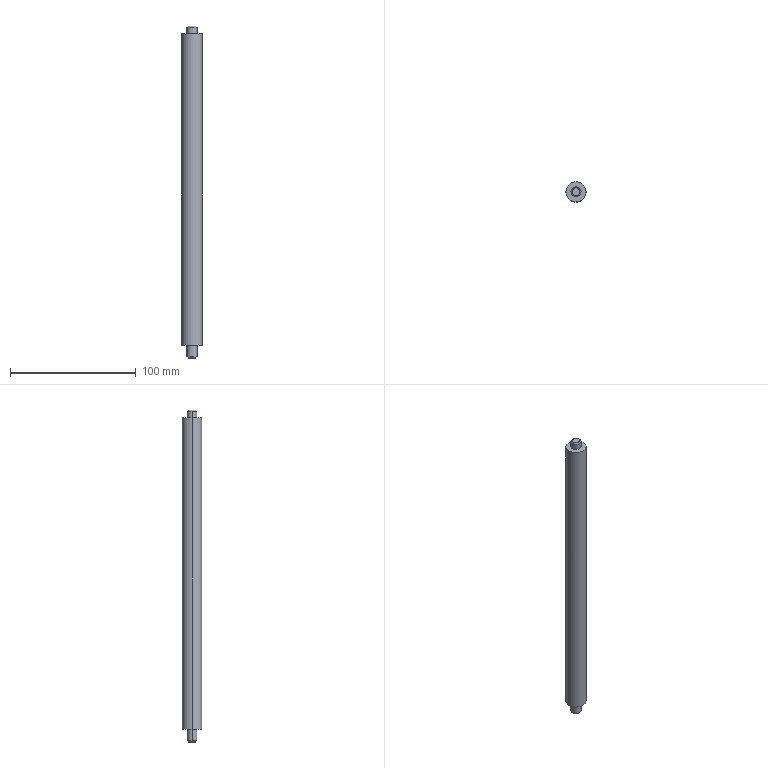Part | SolidWorks | features ICE 2, Chamfer 1, Extrusion 1, Helix 1 | 1 solid | 14 faces | box 16 x 16 x 264 mm | volume 50645 mm3 | cylinder 6 | cone 4 | plane 4 | commonest cylinder face diameters 8 x4 16 x2
STEP:
#1=CARTESIAN_POINT('',(3.,0.,254.));
#2=VERTEX_POINT('',#1);
#3=CARTESIAN_POINT('',(-3.,0.,254.));
#4=VERTEX_POINT('',#3);
#5=CARTESIAN_POINT('',(0.,0.,254.));
#6=DIRECTION('',(0.,0.,1.));
#7=DIRECTION('',(1.,0.,0.));
#8=AXIS2_PLACEMENT_3D('',#5,#6,#7);
#9=CIRCLE('',#8,3.);
#10=EDGE_CURVE('',#2,#4,#9,.T.);
#11=ORIENTED_EDGE('',*,*,#10,.F.);
#12=CARTESIAN_POINT('',(4.,0.,253.));
#13=VERTEX_POINT('',#12);
#14=CARTESIAN_POINT('',(3.,0.,254.));
#15=DIRECTION('',(0.7071,0.,-0.7071));
#16=VECTOR('',#15,1000.);
#17=LINE('',#14,#16);
#18=EDGE_CURVE('',#2,#13,#17,.T.);
#19=ORIENTED_EDGE('',*,*,#18,.T.);
#20=CARTESIAN_POINT('',(-4.,0.,253.));
#21=VERTEX_POINT('',#20);
#22=CARTESIAN_POINT('',(0.,0.,253.));
#23=DIRECTION('',(0.,0.,-1.));
#24=DIRECTION('',(1.,0.,0.));
#25=AXIS2_PLACEMENT_3D('',#22,#23,#24);
#26=CIRCLE('',#25,4.);
#27=EDGE_CURVE('',#21,#13,#26,.T.);
#28=ORIENTED_EDGE('',*,*,#27,.F.);
#29=CARTESIAN_POINT('',(-3.,0.,254.));
#30=DIRECTION('',(-0.7071,0.,-0.7071));
#31=VECTOR('',#30,1000.);
#32=LINE('',#29,#31);
#33=EDGE_CURVE('',#4,#21,#32,.T.);
#34=ORIENTED_EDGE('',*,*,#33,.F.);
#35=EDGE_LOOP('',(#11,#19,#28,#34));
#36=FACE_OUTER_BOUND('',#35,.T.);
#37=CARTESIAN_POINT('',(0.,0.,254.));
#38=DIRECTION('',(0.,0.,-1.));
#39=DIRECTION('',(-1.,0.,0.));
#40=AXIS2_PLACEMENT_3D('',#37,#38,#39);
#41=CONICAL_SURFACE('',#40,3.,0.7854);
#42=ADVANCED_FACE('',(#36),#41,.T.);
#43=CARTESIAN_POINT('',(-3.,0.,-10.));
#44=VERTEX_POINT('',#43);
#45=CARTESIAN_POINT('',(3.,0.,-10.));
#46=VERTEX_POINT('',#45);
#47=CARTESIAN_POINT('',(0.,0.,-10.));
#48=DIRECTION('',(0.,0.,-1.));
#49=DIRECTION('',(-1.,0.,0.));
#50=AXIS2_PLACEMENT_3D('',#47,#48,#49);
#51=CIRCLE('',#50,3.);
#52=EDGE_CURVE('',#44,#46,#51,.T.);
#53=ORIENTED_EDGE('',*,*,#52,.F.);
#54=CARTESIAN_POINT('',(-4.,0.,-9.));
#55=VERTEX_POINT('',#54);
#56=CARTESIAN_POINT('',(-3.,0.,-10.));
#57=DIRECTION('',(-0.7071,0.,0.7071));
#58=VECTOR('',#57,1000.);
#59=LINE('',#56,#58);
#60=EDGE_CURVE('',#44,#55,#59,.T.);
#61=ORIENTED_EDGE('',*,*,#60,.T.);
#62=CARTESIAN_POINT('',(4.,0.,-9.));
#63=VERTEX_POINT('',#62);
#64=CARTESIAN_POINT('',(0.,0.,-9.));
#65=DIRECTION('',(0.,0.,1.));
#66=DIRECTION('',(-1.,0.,0.));
#67=AXIS2_PLACEMENT_3D('',#64,#65,#66);
#68=CIRCLE('',#67,4.);
#69=EDGE_CURVE('',#63,#55,#68,.T.);
#70=ORIENTED_EDGE('',*,*,#69,.F.);
#71=CARTESIAN_POINT('',(3.,0.,-10.));
#72=DIRECTION('',(0.7071,0.,0.7071));
#73=VECTOR('',#72,1000.);
#74=LINE('',#71,#73);
#75=EDGE_CURVE('',#46,#63,#74,.T.);
#76=ORIENTED_EDGE('',*,*,#75,.F.);
#77=EDGE_LOOP('',(#53,#61,#70,#76));
#78=FACE_OUTER_BOUND('',#77,.T.);
#79=CARTESIAN_POINT('',(0.,0.,-10.));
#80=DIRECTION('',(0.,0.,1.));
#81=DIRECTION('',(1.,0.,0.));
#82=AXIS2_PLACEMENT_3D('',#79,#80,#81);
#83=CONICAL_SURFACE('',#82,3.,0.7854);
#84=ADVANCED_FACE('',(#78),#83,.T.);
#85=ORIENTED_EDGE('',*,*,#27,.T.);
#86=CARTESIAN_POINT('',(4.,0.,248.));
#87=VERTEX_POINT('',#86);
#88=CARTESIAN_POINT('',(4.,0.,254.));
#89=DIRECTION('',(0.,0.,-1.));
#90=VECTOR('',#89,1000.);
#91=LINE('',#88,#90);
#92=EDGE_CURVE('',#13,#87,#91,.T.);
#93=ORIENTED_EDGE('',*,*,#92,.T.);
#94=CARTESIAN_POINT('',(-4.,0.,248.));
#95=VERTEX_POINT('',#94);
#96=CARTESIAN_POINT('',(0.,0.,248.));
#97=DIRECTION('',(0.,0.,1.));
#98=DIRECTION('',(1.,0.,0.));
#99=AXIS2_PLACEMENT_3D('',#96,#97,#98);
#100=CIRCLE('',#99,4.);
#101=EDGE_CURVE('',#87,#95,#100,.T.);
#102=ORIENTED_EDGE('',*,*,#101,.T.);
#103=CARTESIAN_POINT('',(-4.,0.,254.));
#104=DIRECTION('',(0.,0.,-1.));
#105=VECTOR('',#104,1000.);
#106=LINE('',#103,#105);
#107=EDGE_CURVE('',#21,#95,#106,.T.);
#108=ORIENTED_EDGE('',*,*,#107,.F.);
#109=EDGE_LOOP('',(#85,#93,#102,#108));
#110=FACE_OUTER_BOUND('',#109,.T.);
#111=CARTESIAN_POINT('',(0.,0.,254.));
#112=DIRECTION('',(0.,0.,-1.));
#113=DIRECTION('',(-1.,0.,0.));
#114=AXIS2_PLACEMENT_3D('',#111,#112,#113);
#115=CYLINDRICAL_SURFACE('',#114,4.);
#116=ADVANCED_FACE('',(#110),#115,.T.);
#117=ORIENTED_EDGE('',*,*,#69,.T.);
#118=CARTESIAN_POINT('',(-4.,0.,0.));
#119=VERTEX_POINT('',#118);
#120=CARTESIAN_POINT('',(-4.,0.,-10.));
#121=DIRECTION('',(0.,0.,1.));
#122=VECTOR('',#121,1000.);
#123=LINE('',#120,#122);
#124=EDGE_CURVE('',#55,#119,#123,.T.);
#125=ORIENTED_EDGE('',*,*,#124,.T.);
#126=CARTESIAN_POINT('',(4.,0.,0.));
#127=VERTEX_POINT('',#126);
#128=CARTESIAN_POINT('',(0.,0.,0.));
#129=DIRECTION('',(0.,0.,-1.));
#130=DIRECTION('',(1.,0.,0.));
#131=AXIS2_PLACEMENT_3D('',#128,#129,#130);
#132=CIRCLE('',#131,4.);
#133=EDGE_CURVE('',#119,#127,#132,.T.);
#134=ORIENTED_EDGE('',*,*,#133,.T.);
#135=CARTESIAN_POINT('',(4.,0.,-10.));
#136=DIRECTION('',(0.,0.,1.));
#137=VECTOR('',#136,1000.);
#138=LINE('',#135,#137);
#139=EDGE_CURVE('',#63,#127,#138,.T.);
#140=ORIENTED_EDGE('',*,*,#139,.F.);
#141=EDGE_LOOP('',(#117,#125,#134,#140));
#142=FACE_OUTER_BOUND('',#141,.T.);
#143=CARTESIAN_POINT('',(0.,0.,-10.));
#144=DIRECTION('',(0.,0.,1.));
#145=DIRECTION('',(1.,0.,0.));
#146=AXIS2_PLACEMENT_3D('',#143,#144,#145);
#147=CYLINDRICAL_SURFACE('',#146,4.);
#148=ADVANCED_FACE('',(#142),#147,.T.);
#149=CARTESIAN_POINT('',(8.,0.,248.));
#150=VERTEX_POINT('',#149);
#151=CARTESIAN_POINT('',(-8.,0.,248.));
#152=VERTEX_POINT('',#151);
#153=CARTESIAN_POINT('',(0.,0.,248.));
#154=DIRECTION('',(0.,0.,1.));
#155=DIRECTION('',(1.,0.,0.));
#156=AXIS2_PLACEMENT_3D('',#153,#154,#155);
#157=CIRCLE('',#156,8.);
#158=EDGE_CURVE('',#150,#152,#157,.T.);
#159=ORIENTED_EDGE('',*,*,#158,.F.);
#160=CARTESIAN_POINT('',(8.,0.,0.));
#161=VERTEX_POINT('',#160);
#162=CARTESIAN_POINT('',(8.,0.,248.));
#163=DIRECTION('',(0.,0.,-1.));
#164=VECTOR('',#163,1000.);
#165=LINE('',#162,#164);
#166=EDGE_CURVE('',#150,#161,#165,.T.);
#167=ORIENTED_EDGE('',*,*,#166,.T.);
#168=CARTESIAN_POINT('',(-8.,0.,0.));
#169=VERTEX_POINT('',#168);
#170=CARTESIAN_POINT('',(0.,0.,0.));
#171=DIRECTION('',(0.,0.,1.));
#172=DIRECTION('',(1.,0.,0.));
#173=AXIS2_PLACEMENT_3D('',#170,#171,#172);
#174=CIRCLE('',#173,8.);
#175=EDGE_CURVE('',#161,#169,#174,.T.);
#176=ORIENTED_EDGE('',*,*,#175,.T.);
#177=CARTESIAN_POINT('',(-8.,0.,248.));
#178=DIRECTION('',(0.,0.,-1.));
#179=VECTOR('',#178,1000.);
#180=LINE('',#177,#179);
#181=EDGE_CURVE('',#152,#169,#180,.T.);
#182=ORIENTED_EDGE('',*,*,#181,.F.);
#183=EDGE_LOOP('',(#159,#167,#176,#182));
#184=FACE_OUTER_BOUND('',#183,.T.);
#185=CARTESIAN_POINT('',(0.,0.,248.));
#186=DIRECTION('',(0.,0.,-1.));
#187=DIRECTION('',(-1.,0.,0.));
#188=AXIS2_PLACEMENT_3D('',#185,#186,#187);
#189=CYLINDRICAL_SURFACE('',#188,8.);
#190=ADVANCED_FACE('',(#184),#189,.T.);
#191=CARTESIAN_POINT('',(0.,0.,248.));
#192=DIRECTION('',(0.,0.,1.));
#193=DIRECTION('',(1.,0.,0.));
#194=AXIS2_PLACEMENT_3D('',#191,#192,#193);
#195=CIRCLE('',#194,8.);
#196=EDGE_CURVE('',#152,#150,#195,.T.);
#197=ORIENTED_EDGE('',*,*,#196,.T.);
#198=ORIENTED_EDGE('',*,*,#158,.T.);
#199=EDGE_LOOP('',(#197,#198));
#200=FACE_OUTER_BOUND('',#199,.T.);
#201=CARTESIAN_POINT('',(0.,0.,248.));
#202=DIRECTION('',(0.,0.,1.));
#203=DIRECTION('',(1.,0.,0.));
#204=AXIS2_PLACEMENT_3D('',#201,#202,#203);
#205=CIRCLE('',#204,4.);
#206=EDGE_CURVE('',#95,#87,#205,.T.);
#207=ORIENTED_EDGE('',*,*,#206,.F.);
#208=ORIENTED_EDGE('',*,*,#101,.F.);
#209=EDGE_LOOP('',(#207,#208));
#210=FACE_BOUND('',#209,.T.);
#211=CARTESIAN_POINT('',(0.,0.,248.));
#212=DIRECTION('',(0.,0.,1.));
#213=DIRECTION('',(1.,0.,0.));
#214=AXIS2_PLACEMENT_3D('',#211,#212,#213);
#215=PLANE('',#214);
#216=ADVANCED_FACE('',(#200,#210),#215,.T.);
#217=CARTESIAN_POINT('',(0.,0.,0.));
#218=DIRECTION('',(0.,0.,1.));
#219=DIRECTION('',(1.,0.,0.));
#220=AXIS2_PLACEMENT_3D('',#217,#218,#219);
#221=CIRCLE('',#220,8.);
#222=EDGE_CURVE('',#169,#161,#221,.T.);
#223=ORIENTED_EDGE('',*,*,#222,.F.);
#224=ORIENTED_EDGE('',*,*,#175,.F.);
#225=EDGE_LOOP('',(#223,#224));
#226=FACE_OUTER_BOUND('',#225,.T.);
#227=CARTESIAN_POINT('',(0.,0.,0.));
#228=DIRECTION('',(0.,0.,-1.));
#229=DIRECTION('',(1.,0.,0.));
#230=AXIS2_PLACEMENT_3D('',#227,#228,#229);
#231=CIRCLE('',#230,4.);
#232=EDGE_CURVE('',#127,#119,#231,.T.);
#233=ORIENTED_EDGE('',*,*,#232,.F.);
#234=ORIENTED_EDGE('',*,*,#133,.F.);
#235=EDGE_LOOP('',(#233,#234));
#236=FACE_BOUND('',#235,.T.);
#237=CARTESIAN_POINT('',(0.,0.,0.));
#238=DIRECTION('',(0.,0.,1.));
#239=DIRECTION('',(1.,0.,0.));
#240=AXIS2_PLACEMENT_3D('',#237,#238,#239);
#241=PLANE('',#240);
#242=ADVANCED_FACE('',(#226,#236),#241,.F.);
#243=ORIENTED_EDGE('',*,*,#166,.F.);
#244=ORIENTED_EDGE('',*,*,#196,.F.);
#245=ORIENTED_EDGE('',*,*,#181,.T.);
#246=ORIENTED_EDGE('',*,*,#222,.T.);
#247=EDGE_LOOP('',(#243,#244,#245,#246));
#248=FACE_OUTER_BOUND('',#247,.T.);
#249=CARTESIAN_POINT('',(0.,0.,248.));
#250=DIRECTION('',(0.,0.,-1.));
#251=DIRECTION('',(-1.,0.,0.));
#252=AXIS2_PLACEMENT_3D('',#249,#250,#251);
#253=CYLINDRICAL_SURFACE('',#252,8.);
#254=ADVANCED_FACE('',(#248),#253,.T.);
#255=ORIENTED_EDGE('',*,*,#124,.F.);
#256=CARTESIAN_POINT('',(0.,0.,-9.));
#257=DIRECTION('',(0.,0.,1.));
#258=DIRECTION('',(-1.,0.,0.));
#259=AXIS2_PLACEMENT_3D('',#256,#257,#258);
#260=CIRCLE('',#259,4.);
#261=EDGE_CURVE('',#55,#63,#260,.T.);
#262=ORIENTED_EDGE('',*,*,#261,.T.);
#263=ORIENTED_EDGE('',*,*,#139,.T.);
#264=ORIENTED_EDGE('',*,*,#232,.T.);
#265=EDGE_LOOP('',(#255,#262,#263,#264));
#266=FACE_OUTER_BOUND('',#265,.T.);
#267=CARTESIAN_POINT('',(0.,0.,-10.));
#268=DIRECTION('',(0.,0.,1.));
#269=DIRECTION('',(1.,0.,0.));
#270=AXIS2_PLACEMENT_3D('',#267,#268,#269);
#271=CYLINDRICAL_SURFACE('',#270,4.);
#272=ADVANCED_FACE('',(#266),#271,.T.);
#273=CARTESIAN_POINT('',(0.,0.,-10.));
#274=DIRECTION('',(0.,0.,-1.));
#275=DIRECTION('',(-1.,0.,0.));
#276=AXIS2_PLACEMENT_3D('',#273,#274,#275);
#277=CIRCLE('',#276,3.);
#278=EDGE_CURVE('',#46,#44,#277,.T.);
#279=ORIENTED_EDGE('',*,*,#278,.T.);
#280=ORIENTED_EDGE('',*,*,#52,.T.);
#281=EDGE_LOOP('',(#279,#280));
#282=FACE_OUTER_BOUND('',#281,.T.);
#283=CARTESIAN_POINT('',(0.,0.,-10.));
#284=DIRECTION('',(0.,0.,-1.));
#285=DIRECTION('',(-1.,0.,0.));
#286=AXIS2_PLACEMENT_3D('',#283,#284,#285);
#287=PLANE('',#286);
#288=ADVANCED_FACE('',(#282),#287,.T.);
#289=ORIENTED_EDGE('',*,*,#92,.F.);
#290=CARTESIAN_POINT('',(0.,0.,253.));
#291=DIRECTION('',(0.,0.,-1.));
#292=DIRECTION('',(1.,0.,0.));
#293=AXIS2_PLACEMENT_3D('',#290,#291,#292);
#294=CIRCLE('',#293,4.);
#295=EDGE_CURVE('',#13,#21,#294,.T.);
#296=ORIENTED_EDGE('',*,*,#295,.T.);
#297=ORIENTED_EDGE('',*,*,#107,.T.);
#298=ORIENTED_EDGE('',*,*,#206,.T.);
#299=EDGE_LOOP('',(#289,#296,#297,#298));
#300=FACE_OUTER_BOUND('',#299,.T.);
#301=CARTESIAN_POINT('',(0.,0.,254.));
#302=DIRECTION('',(0.,0.,-1.));
#303=DIRECTION('',(-1.,0.,0.));
#304=AXIS2_PLACEMENT_3D('',#301,#302,#303);
#305=CYLINDRICAL_SURFACE('',#304,4.);
#306=ADVANCED_FACE('',(#300),#305,.T.);
#307=CARTESIAN_POINT('',(0.,0.,254.));
#308=DIRECTION('',(0.,0.,1.));
#309=DIRECTION('',(1.,0.,0.));
#310=AXIS2_PLACEMENT_3D('',#307,#308,#309);
#311=CIRCLE('',#310,3.);
#312=EDGE_CURVE('',#4,#2,#311,.T.);
#313=ORIENTED_EDGE('',*,*,#312,.T.);
#314=ORIENTED_EDGE('',*,*,#10,.T.);
#315=EDGE_LOOP('',(#313,#314));
#316=FACE_OUTER_BOUND('',#315,.T.);
#317=CARTESIAN_POINT('',(0.,0.,254.));
#318=DIRECTION('',(0.,0.,1.));
#319=DIRECTION('',(1.,0.,0.));
#320=AXIS2_PLACEMENT_3D('',#317,#318,#319);
#321=PLANE('',#320);
#322=ADVANCED_FACE('',(#316),#321,.T.);
#323=ORIENTED_EDGE('',*,*,#60,.F.);
#324=ORIENTED_EDGE('',*,*,#278,.F.);
#325=ORIENTED_EDGE('',*,*,#75,.T.);
#326=ORIENTED_EDGE('',*,*,#261,.F.);
#327=EDGE_LOOP('',(#323,#324,#325,#326));
#328=FACE_OUTER_BOUND('',#327,.T.);
#329=CARTESIAN_POINT('',(0.,0.,-10.));
#330=DIRECTION('',(0.,0.,1.));
#331=DIRECTION('',(1.,0.,0.));
#332=AXIS2_PLACEMENT_3D('',#329,#330,#331);
#333=CONICAL_SURFACE('',#332,3.,0.7854);
#334=ADVANCED_FACE('',(#328),#333,.T.);
#335=ORIENTED_EDGE('',*,*,#18,.F.);
#336=ORIENTED_EDGE('',*,*,#312,.F.);
#337=ORIENTED_EDGE('',*,*,#33,.T.);
#338=ORIENTED_EDGE('',*,*,#295,.F.);
#339=EDGE_LOOP('',(#335,#336,#337,#338));
#340=FACE_OUTER_BOUND('',#339,.T.);
#341=CARTESIAN_POINT('',(0.,0.,254.));
#342=DIRECTION('',(0.,0.,-1.));
#343=DIRECTION('',(-1.,0.,0.));
#344=AXIS2_PLACEMENT_3D('',#341,#342,#343);
#345=CONICAL_SURFACE('',#344,3.,0.7854);
#346=ADVANCED_FACE('',(#340),#345,.T.);
#347=CLOSED_SHELL('',(#42,#84,#116,#148,#190,#216,#242,#254,#272,#288,#306,#322,#334,#346));
#348=MANIFOLD_SOLID_BREP('',#347);
#349=CARTESIAN_POINT('',(0.,0.,0.));
#350=DIRECTION('',(0.,0.,1.));
#351=DIRECTION('',(1.,0.,0.));
#352=AXIS2_PLACEMENT_3D('',#349,#350,#351);
#353=(LENGTH_UNIT()NAMED_UNIT(*)SI_UNIT(.MILLI.,.METRE.));
#354=UNCERTAINTY_MEASURE_WITH_UNIT(LENGTH_MEASURE(0.00001),#353,'','');
#355=(NAMED_UNIT(*)PLANE_ANGLE_UNIT()SI_UNIT($,.RADIAN.));
#356=(NAMED_UNIT(*)SI_UNIT($,.STERADIAN.)SOLID_ANGLE_UNIT());
#357=(GEOMETRIC_REPRESENTATION_CONTEXT(3)GLOBAL_UNCERTAINTY_ASSIGNED_CONTEXT((#354))GLOBAL_UNIT_ASSIGNED_CONTEXT((#353,#355,#356))REPRESENTATION_CONTEXT('',''));
#358=ADVANCED_BREP_SHAPE_REPRESENTATION('',(#348,#352),#357);